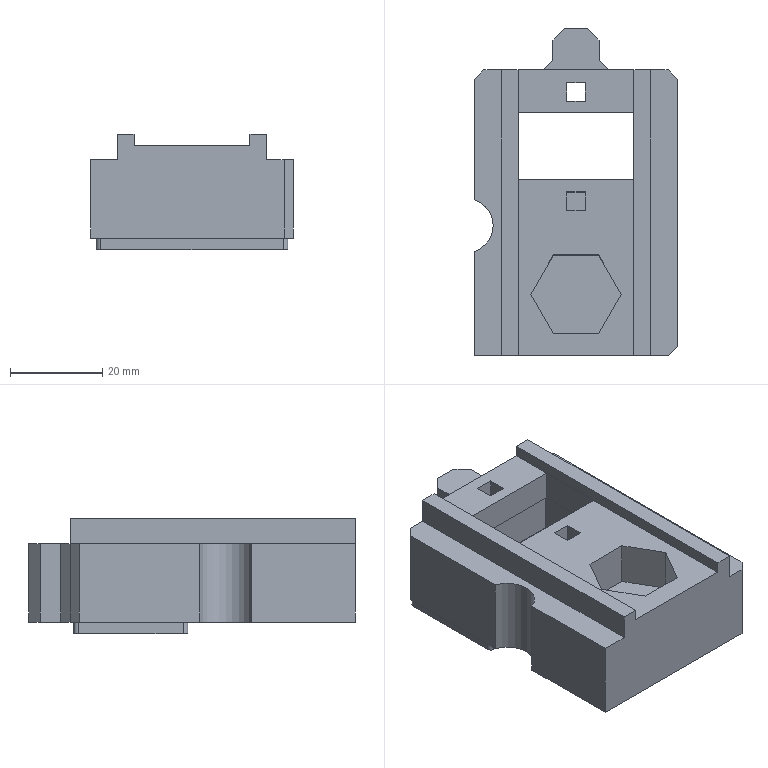Part | STEP file | 58413461 | 1 solid | 96 faces | box 44 x 71 x 25 mm | volume 30731 mm3 | plane 86 | cylinder 10 | commonest cylinder face diameters 2 x8 12 x1 18 x1